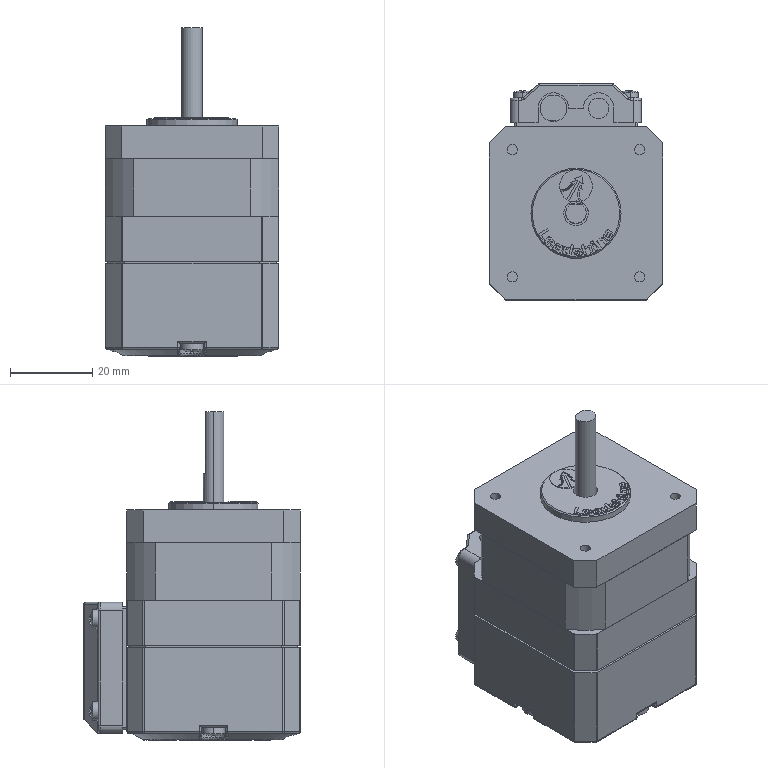Part | STEP file | 42CME02^FBDS-CS | 27 solids | 4144 faces | volume 53634 mm3 | cone 1297 | plane 1228 | cylinder 1155 | spline 414 | sphere 34 | torus 16 | commonest cylinder face diameters 3 x408 2.5 x290 1 x64 0.6 x62 26 x33 14.011 x25